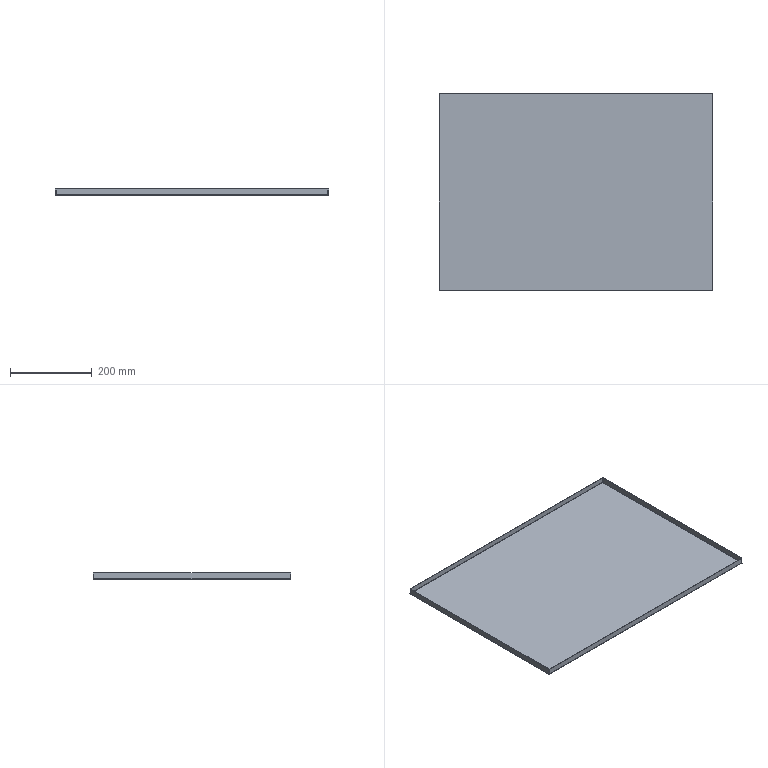Part | SolidWorks | 1 solid | 38 faces | box 670.001 x 485.001 x 15 mm | volume 532568 mm3 | plane 22 | spline 8 | cylinder 8 | commonest cylinder face diameters 0.2 x4 3.2 x4
STEP:
#1=CARTESIAN_POINT('',(333.4,-240.9,-1.5));
#2=VERTEX_POINT('',#1);
#3=CARTESIAN_POINT('',(-333.4,-240.9,-1.5));
#4=VERTEX_POINT('',#3);
#5=CARTESIAN_POINT('',(333.4,-240.9,-1.5));
#6=DIRECTION('',(-1.,0.,0.));
#7=VECTOR('',#6,1000.);
#8=LINE('',#5,#7);
#9=EDGE_CURVE('',#2,#4,#8,.T.);
#10=ORIENTED_EDGE('',*,*,#9,.T.);
#11=CARTESIAN_POINT('',(-333.4,240.9,-1.5));
#12=VERTEX_POINT('',#11);
#13=CARTESIAN_POINT('',(-333.4,-240.9,-1.5));
#14=DIRECTION('',(0.,1.,0.));
#15=VECTOR('',#14,1000.);
#16=LINE('',#13,#15);
#17=EDGE_CURVE('',#4,#12,#16,.T.);
#18=ORIENTED_EDGE('',*,*,#17,.T.);
#19=CARTESIAN_POINT('',(333.4,240.9,-1.5));
#20=VERTEX_POINT('',#19);
#21=CARTESIAN_POINT('',(-333.4,240.9,-1.5));
#22=DIRECTION('',(1.,0.,0.));
#23=VECTOR('',#22,1000.);
#24=LINE('',#21,#23);
#25=EDGE_CURVE('',#12,#20,#24,.T.);
#26=ORIENTED_EDGE('',*,*,#25,.T.);
#27=CARTESIAN_POINT('',(333.4,240.9,-1.5));
#28=DIRECTION('',(0.,-1.,0.));
#29=VECTOR('',#28,1000.);
#30=LINE('',#27,#29);
#31=EDGE_CURVE('',#20,#2,#30,.T.);
#32=ORIENTED_EDGE('',*,*,#31,.T.);
#33=EDGE_LOOP('',(#10,#18,#26,#32));
#34=FACE_OUTER_BOUND('',#33,.T.);
#35=CARTESIAN_POINT('',(0.,0.,-1.5));
#36=DIRECTION('',(0.,0.,1.));
#37=DIRECTION('',(1.,0.,0.));
#38=AXIS2_PLACEMENT_3D('',#35,#36,#37);
#39=PLANE('',#38);
#40=ADVANCED_FACE('',(#34),#39,.F.);
#41=CARTESIAN_POINT('',(-333.4,-240.9,0.));
#42=VERTEX_POINT('',#41);
#43=CARTESIAN_POINT('',(-333.4,240.9,0.));
#44=VERTEX_POINT('',#43);
#45=CARTESIAN_POINT('',(-333.4,-240.9,0.));
#46=DIRECTION('',(0.,1.,0.));
#47=VECTOR('',#46,1000.);
#48=LINE('',#45,#47);
#49=EDGE_CURVE('',#42,#44,#48,.T.);
#50=ORIENTED_EDGE('',*,*,#49,.F.);
#51=CARTESIAN_POINT('',(333.4,-240.9,0.));
#52=VERTEX_POINT('',#51);
#53=CARTESIAN_POINT('',(333.4,-240.9,0.));
#54=DIRECTION('',(-1.,0.,0.));
#55=VECTOR('',#54,1000.);
#56=LINE('',#53,#55);
#57=EDGE_CURVE('',#52,#42,#56,.T.);
#58=ORIENTED_EDGE('',*,*,#57,.F.);
#59=CARTESIAN_POINT('',(333.4,240.9,0.));
#60=VERTEX_POINT('',#59);
#61=CARTESIAN_POINT('',(333.4,240.9,0.));
#62=DIRECTION('',(0.,-1.,0.));
#63=VECTOR('',#62,1000.);
#64=LINE('',#61,#63);
#65=EDGE_CURVE('',#60,#52,#64,.T.);
#66=ORIENTED_EDGE('',*,*,#65,.F.);
#67=CARTESIAN_POINT('',(-333.4,240.9,0.));
#68=DIRECTION('',(1.,0.,0.));
#69=VECTOR('',#68,1000.);
#70=LINE('',#67,#69);
#71=EDGE_CURVE('',#44,#60,#70,.T.);
#72=ORIENTED_EDGE('',*,*,#71,.F.);
#73=EDGE_LOOP('',(#50,#58,#66,#72));
#74=FACE_OUTER_BOUND('',#73,.T.);
#75=CARTESIAN_POINT('',(0.,0.,0.));
#76=DIRECTION('',(0.,0.,1.));
#77=DIRECTION('',(1.,0.,0.));
#78=AXIS2_PLACEMENT_3D('',#75,#76,#77);
#79=PLANE('',#78);
#80=ADVANCED_FACE('',(#74),#79,.T.);
#81=CARTESIAN_POINT('',(-335.,240.293,0.1));
#82=VERTEX_POINT('',#81);
#83=CARTESIAN_POINT('',(-333.5,240.293,0.1));
#84=VERTEX_POINT('',#83);
#85=CARTESIAN_POINT('',(-333.5,240.293,0.1));
#86=DIRECTION('',(1.,0.,0.));
#87=VECTOR('',#86,1000.);
#88=LINE('',#85,#87);
#89=EDGE_CURVE('',#82,#84,#88,.T.);
#90=ORIENTED_EDGE('',*,*,#89,.T.);
#91=CARTESIAN_POINT('',(-333.4,240.9,0.));
#92=CARTESIAN_POINT('',(-333.426,240.799,0.));
#93=CARTESIAN_POINT('',(-333.452,240.698,0.01078));
#94=CARTESIAN_POINT('',(-333.489,240.495,0.0478));
#95=CARTESIAN_POINT('',(-333.5,240.394,0.07382));
#96=CARTESIAN_POINT('',(-333.5,240.293,0.1));
#97=B_SPLINE_CURVE_WITH_KNOTS('',3,(#91,#92,#93,#94,#95,#96),.UNSPECIFIED.,.F.,.F.,(4,2,4),(0.,0.5,1.),.UNSPECIFIED.);
#98=EDGE_CURVE('',#44,#84,#97,.T.);
#99=ORIENTED_EDGE('',*,*,#98,.F.);
#100=CARTESIAN_POINT('',(-333.4,240.9,0.));
#101=DIRECTION('',(0.,0.,-1.));
#102=VECTOR('',#101,1000.);
#103=LINE('',#100,#102);
#104=EDGE_CURVE('',#44,#12,#103,.T.);
#105=ORIENTED_EDGE('',*,*,#104,.T.);
#106=CARTESIAN_POINT('',(-333.4,240.9,-1.5));
#107=CARTESIAN_POINT('',(-333.612,240.849,-1.5));
#108=CARTESIAN_POINT('',(-333.815,240.8,-1.46));
#109=CARTESIAN_POINT('',(-334.205,240.698,-1.299));
#110=CARTESIAN_POINT('',(-334.381,240.648,-1.181));
#111=CARTESIAN_POINT('',(-334.605,240.571,-0.9582));
#112=CARTESIAN_POINT('',(-334.671,240.546,-0.8775));
#113=CARTESIAN_POINT('',(-334.787,240.496,-0.7041));
#114=CARTESIAN_POINT('',(-334.838,240.47,-0.6103));
#115=CARTESIAN_POINT('',(-334.958,240.394,-0.32));
#116=CARTESIAN_POINT('',(-335.,240.344,-0.1115));
#117=CARTESIAN_POINT('',(-335.,240.293,0.1));
#118=B_SPLINE_CURVE_WITH_KNOTS('',3,(#106,#107,#108,#109,#110,#111,#112,#113,#114,#115,#116,#117),.UNSPECIFIED.,.F.,.F.,(4,2,2,2,2,4),(0.,0.0006399,0.00128,0.0016,0.00192,0.00256),.UNSPECIFIED.);
#119=EDGE_CURVE('',#12,#82,#118,.T.);
#120=ORIENTED_EDGE('',*,*,#119,.T.);
#121=EDGE_LOOP('',(#90,#99,#105,#120));
#122=FACE_OUTER_BOUND('',#121,.T.);
#123=CARTESIAN_POINT('',(-333.4,240.9,-1.515));
#124=CARTESIAN_POINT('',(-333.611,240.849,-1.515));
#125=CARTESIAN_POINT('',(-333.823,240.799,-1.473));
#126=CARTESIAN_POINT('',(-334.213,240.698,-1.311));
#127=CARTESIAN_POINT('',(-334.392,240.647,-1.191));
#128=CARTESIAN_POINT('',(-334.691,240.546,-0.8925));
#129=CARTESIAN_POINT('',(-334.811,240.495,-0.7133));
#130=CARTESIAN_POINT('',(-334.973,240.394,-0.3227));
#131=CARTESIAN_POINT('',(-335.015,240.343,-0.1114));
#132=CARTESIAN_POINT('',(-335.015,240.293,0.1));
#133=CARTESIAN_POINT('',(-333.4,240.9,-1.5));
#134=CARTESIAN_POINT('',(-333.609,240.849,-1.5));
#135=CARTESIAN_POINT('',(-333.819,240.799,-1.458));
#136=CARTESIAN_POINT('',(-334.206,240.698,-1.298));
#137=CARTESIAN_POINT('',(-334.383,240.647,-1.179));
#138=CARTESIAN_POINT('',(-334.679,240.546,-0.8833));
#139=CARTESIAN_POINT('',(-334.798,240.495,-0.7058));
#140=CARTESIAN_POINT('',(-334.958,240.394,-0.3188));
#141=CARTESIAN_POINT('',(-335.,240.343,-0.1095));
#142=CARTESIAN_POINT('',(-335.,240.293,0.1));
#143=CARTESIAN_POINT('',(-333.4,240.9,0.));
#144=CARTESIAN_POINT('',(-333.413,240.849,0.));
#145=CARTESIAN_POINT('',(-333.426,240.799,0.002603));
#146=CARTESIAN_POINT('',(-333.45,240.698,0.01262));
#147=CARTESIAN_POINT('',(-333.461,240.647,0.02003));
#148=CARTESIAN_POINT('',(-333.48,240.546,0.03855));
#149=CARTESIAN_POINT('',(-333.487,240.495,0.04964));
#150=CARTESIAN_POINT('',(-333.497,240.394,0.07383));
#151=CARTESIAN_POINT('',(-333.5,240.343,0.08691));
#152=CARTESIAN_POINT('',(-333.5,240.293,0.1));
#153=B_SPLINE_SURFACE_WITH_KNOTS('',1,3,((#123,#124,#125,#126,#127,#128,#129,#130,#131,#132),(#133,#134,#135,#136,#137,#138,#139,#140,#141,#142),(#143,#144,#145,#146,#147,#148,#149,#150,#151,#152)),.UNSPECIFIED.,.F.,.F.,.F.,(2,1,2),(4,2,2,2,4),(-0.01,0.,1.),(0.,0.25,0.5,0.75,1.),.UNSPECIFIED.);
#154=ADVANCED_FACE('',(#122),#153,.F.);
#155=CARTESIAN_POINT('',(-333.5,-240.293,0.1));
#156=VERTEX_POINT('',#155);
#157=CARTESIAN_POINT('',(-333.5,-240.293,0.1));
#158=CARTESIAN_POINT('',(-333.5,-240.394,0.07382));
#159=CARTESIAN_POINT('',(-333.489,-240.495,0.0478));
#160=CARTESIAN_POINT('',(-333.452,-240.698,0.01078));
#161=CARTESIAN_POINT('',(-333.426,-240.799,0.));
#162=CARTESIAN_POINT('',(-333.4,-240.9,0.));
#163=B_SPLINE_CURVE_WITH_KNOTS('',3,(#157,#158,#159,#160,#161,#162),.UNSPECIFIED.,.F.,.F.,(4,2,4),(0.,0.5,1.),.UNSPECIFIED.);
#164=EDGE_CURVE('',#156,#42,#163,.T.);
#165=ORIENTED_EDGE('',*,*,#164,.F.);
#166=CARTESIAN_POINT('',(-335.,-240.293,0.1));
#167=VERTEX_POINT('',#166);
#168=CARTESIAN_POINT('',(-333.5,-240.293,0.1));
#169=DIRECTION('',(1.,0.,0.));
#170=VECTOR('',#169,1000.);
#171=LINE('',#168,#170);
#172=EDGE_CURVE('',#167,#156,#171,.T.);
#173=ORIENTED_EDGE('',*,*,#172,.F.);
#174=CARTESIAN_POINT('',(-335.,-240.293,0.1));
#175=CARTESIAN_POINT('',(-335.,-240.344,-0.1115));
#176=CARTESIAN_POINT('',(-334.96,-240.393,-0.3151));
#177=CARTESIAN_POINT('',(-334.799,-240.495,-0.7048));
#178=CARTESIAN_POINT('',(-334.681,-240.545,-0.881));
#179=CARTESIAN_POINT('',(-334.458,-240.621,-1.105));
#180=CARTESIAN_POINT('',(-334.378,-240.647,-1.171));
#181=CARTESIAN_POINT('',(-334.204,-240.697,-1.287));
#182=CARTESIAN_POINT('',(-334.11,-240.723,-1.338));
#183=CARTESIAN_POINT('',(-333.82,-240.799,-1.458));
#184=CARTESIAN_POINT('',(-333.612,-240.849,-1.5));
#185=CARTESIAN_POINT('',(-333.4,-240.9,-1.5));
#186=B_SPLINE_CURVE_WITH_KNOTS('',3,(#174,#175,#176,#177,#178,#179,#180,#181,#182,#183,#184,#185),.UNSPECIFIED.,.F.,.F.,(4,2,2,2,2,4),(0.,0.0006399,0.00128,0.0016,0.00192,0.00256),.UNSPECIFIED.);
#187=EDGE_CURVE('',#167,#4,#186,.T.);
#188=ORIENTED_EDGE('',*,*,#187,.T.);
#189=CARTESIAN_POINT('',(-333.4,-240.9,0.));
#190=DIRECTION('',(0.,0.,-1.));
#191=VECTOR('',#190,1000.);
#192=LINE('',#189,#191);
#193=EDGE_CURVE('',#42,#4,#192,.T.);
#194=ORIENTED_EDGE('',*,*,#193,.F.);
#195=EDGE_LOOP('',(#165,#173,#188,#194));
#196=FACE_OUTER_BOUND('',#195,.T.);
#197=CARTESIAN_POINT('',(-335.015,-240.293,0.1));
#198=CARTESIAN_POINT('',(-335.015,-240.343,-0.1114));
#199=CARTESIAN_POINT('',(-334.973,-240.394,-0.3227));
#200=CARTESIAN_POINT('',(-334.811,-240.495,-0.7133));
#201=CARTESIAN_POINT('',(-334.691,-240.546,-0.8925));
#202=CARTESIAN_POINT('',(-334.392,-240.647,-1.191));
#203=CARTESIAN_POINT('',(-334.213,-240.698,-1.311));
#204=CARTESIAN_POINT('',(-333.823,-240.799,-1.473));
#205=CARTESIAN_POINT('',(-333.611,-240.849,-1.515));
#206=CARTESIAN_POINT('',(-333.4,-240.9,-1.515));
#207=CARTESIAN_POINT('',(-335.,-240.293,0.1));
#208=CARTESIAN_POINT('',(-335.,-240.343,-0.1095));
#209=CARTESIAN_POINT('',(-334.958,-240.394,-0.3188));
#210=CARTESIAN_POINT('',(-334.798,-240.495,-0.7058));
#211=CARTESIAN_POINT('',(-334.679,-240.546,-0.8833));
#212=CARTESIAN_POINT('',(-334.383,-240.647,-1.179));
#213=CARTESIAN_POINT('',(-334.206,-240.698,-1.298));
#214=CARTESIAN_POINT('',(-333.819,-240.799,-1.458));
#215=CARTESIAN_POINT('',(-333.609,-240.849,-1.5));
#216=CARTESIAN_POINT('',(-333.4,-240.9,-1.5));
#217=CARTESIAN_POINT('',(-333.5,-240.293,0.1));
#218=CARTESIAN_POINT('',(-333.5,-240.343,0.08691));
#219=CARTESIAN_POINT('',(-333.497,-240.394,0.07383));
#220=CARTESIAN_POINT('',(-333.487,-240.495,0.04964));
#221=CARTESIAN_POINT('',(-333.48,-240.546,0.03855));
#222=CARTESIAN_POINT('',(-333.461,-240.647,0.02003));
#223=CARTESIAN_POINT('',(-333.45,-240.698,0.01262));
#224=CARTESIAN_POINT('',(-333.426,-240.799,0.002603));
#225=CARTESIAN_POINT('',(-333.413,-240.849,0.));
#226=CARTESIAN_POINT('',(-333.4,-240.9,0.));
#227=B_SPLINE_SURFACE_WITH_KNOTS('',1,3,((#197,#198,#199,#200,#201,#202,#203,#204,#205,#206),(#207,#208,#209,#210,#211,#212,#213,#214,#215,#216),(#217,#218,#219,#220,#221,#222,#223,#224,#225,#226)),.UNSPECIFIED.,.F.,.F.,.F.,(2,1,2),(4,2,2,2,4),(-0.01,0.,1.),(0.,0.25,0.5,0.75,1.),.UNSPECIFIED.);
#228=ADVANCED_FACE('',(#196),#227,.F.);
#229=ORIENTED_EDGE('',*,*,#17,.F.);
#230=ORIENTED_EDGE('',*,*,#187,.F.);
#231=CARTESIAN_POINT('',(-335.,242.5,0.1));
#232=DIRECTION('',(0.,1.,0.));
#233=VECTOR('',#232,1000.);
#234=LINE('',#231,#233);
#235=EDGE_CURVE('',#167,#82,#234,.T.);
#236=ORIENTED_EDGE('',*,*,#235,.T.);
#237=ORIENTED_EDGE('',*,*,#119,.F.);
#238=EDGE_LOOP('',(#229,#230,#236,#237));
#239=FACE_OUTER_BOUND('',#238,.T.);
#240=CARTESIAN_POINT('',(-333.4,-240.9,0.1));
#241=DIRECTION('',(0.,-1.,0.));
#242=DIRECTION('',(-1.,0.,0.));
#243=AXIS2_PLACEMENT_3D('',#240,#241,#242);
#244=CYLINDRICAL_SURFACE('',#243,1.6);
#245=ADVANCED_FACE('',(#239),#244,.T.);
#246=ORIENTED_EDGE('',*,*,#49,.T.);
#247=ORIENTED_EDGE('',*,*,#98,.T.);
#248=CARTESIAN_POINT('',(-333.5,242.5,0.1));
#249=DIRECTION('',(0.,-1.,0.));
#250=VECTOR('',#249,1000.);
#251=LINE('',#248,#250);
#252=EDGE_CURVE('',#84,#156,#251,.T.);
#253=ORIENTED_EDGE('',*,*,#252,.T.);
#254=ORIENTED_EDGE('',*,*,#164,.T.);
#255=EDGE_LOOP('',(#246,#247,#253,#254));
#256=FACE_OUTER_BOUND('',#255,.T.);
#257=CARTESIAN_POINT('',(-333.4,-240.9,0.1));
#258=DIRECTION('',(0.,-1.,0.));
#259=DIRECTION('',(-1.,0.,0.));
#260=AXIS2_PLACEMENT_3D('',#257,#258,#259);
#261=CYLINDRICAL_SURFACE('',#260,0.1);
#262=ADVANCED_FACE('',(#256),#261,.F.);
#263=CARTESIAN_POINT('',(-335.,240.293,13.5));
#264=VERTEX_POINT('',#263);
#265=CARTESIAN_POINT('',(-335.,240.293,0.));
#266=DIRECTION('',(0.,0.,1.));
#267=VECTOR('',#266,1000.);
#268=LINE('',#265,#267);
#269=EDGE_CURVE('',#82,#264,#268,.T.);
#270=ORIENTED_EDGE('',*,*,#269,.T.);
#271=CARTESIAN_POINT('',(-333.5,240.293,13.5));
#272=VERTEX_POINT('',#271);
#273=CARTESIAN_POINT('',(-333.5,240.293,13.5));
#274=DIRECTION('',(1.,0.,0.));
#275=VECTOR('',#274,1000.);
#276=LINE('',#273,#275);
#277=EDGE_CURVE('',#264,#272,#276,.T.);
#278=ORIENTED_EDGE('',*,*,#277,.T.);
#279=CARTESIAN_POINT('',(-333.5,240.293,0.));
#280=DIRECTION('',(0.,0.,1.));
#281=VECTOR('',#280,1000.);
#282=LINE('',#279,#281);
#283=EDGE_CURVE('',#84,#272,#282,.T.);
#284=ORIENTED_EDGE('',*,*,#283,.F.);
#285=ORIENTED_EDGE('',*,*,#89,.F.);
#286=EDGE_LOOP('',(#270,#278,#284,#285));
#287=FACE_OUTER_BOUND('',#286,.T.);
#288=CARTESIAN_POINT('',(-333.5,240.293,0.));
#289=DIRECTION('',(0.,1.,0.));
#290=DIRECTION('',(0.,0.,1.));
#291=AXIS2_PLACEMENT_3D('',#288,#289,#290);
#292=PLANE('',#291);
#293=ADVANCED_FACE('',(#287),#292,.T.);
#294=ORIENTED_EDGE('',*,*,#235,.F.);
#295=CARTESIAN_POINT('',(-335.,-240.293,13.5));
#296=VERTEX_POINT('',#295);
#297=CARTESIAN_POINT('',(-335.,-240.293,0.));
#298=DIRECTION('',(0.,0.,1.));
#299=VECTOR('',#298,1000.);
#300=LINE('',#297,#299);
#301=EDGE_CURVE('',#167,#296,#300,.T.);
#302=ORIENTED_EDGE('',*,*,#301,.T.);
#303=CARTESIAN_POINT('',(-335.,0.,13.5));
#304=DIRECTION('',(0.,1.,0.));
#305=VECTOR('',#304,1000.);
#306=LINE('',#303,#305);
#307=EDGE_CURVE('',#296,#264,#306,.T.);
#308=ORIENTED_EDGE('',*,*,#307,.T.);
#309=ORIENTED_EDGE('',*,*,#269,.F.);
#310=EDGE_LOOP('',(#294,#302,#308,#309));
#311=FACE_OUTER_BOUND('',#310,.T.);
#312=CARTESIAN_POINT('',(-335.,0.,0.));
#313=DIRECTION('',(1.,0.,0.));
#314=DIRECTION('',(0.,0.,-1.));
#315=AXIS2_PLACEMENT_3D('',#312,#313,#314);
#316=PLANE('',#315);
#317=ADVANCED_FACE('',(#311),#316,.F.);
#318=CARTESIAN_POINT('',(-333.5,-240.293,13.5));
#319=VERTEX_POINT('',#318);
#320=CARTESIAN_POINT('',(-333.5,-240.293,0.));
#321=DIRECTION('',(0.,0.,1.));
#322=VECTOR('',#321,1000.);
#323=LINE('',#320,#322);
#324=EDGE_CURVE('',#156,#319,#323,.T.);
#325=ORIENTED_EDGE('',*,*,#324,.F.);
#326=ORIENTED_EDGE('',*,*,#252,.F.);
#327=ORIENTED_EDGE('',*,*,#283,.T.);
#328=CARTESIAN_POINT('',(-333.5,242.5,13.5));
#329=DIRECTION('',(0.,1.,0.));
#330=VECTOR('',#329,1000.);
#331=LINE('',#328,#330);
#332=EDGE_CURVE('',#319,#272,#331,.T.);
#333=ORIENTED_EDGE('',*,*,#332,.F.);
#334=EDGE_LOOP('',(#325,#326,#327,#333));
#335=FACE_OUTER_BOUND('',#334,.T.);
#336=CARTESIAN_POINT('',(-333.5,0.,0.));
#337=DIRECTION('',(1.,0.,0.));
#338=DIRECTION('',(0.,0.,-1.));
#339=AXIS2_PLACEMENT_3D('',#336,#337,#338);
#340=PLANE('',#339);
#341=ADVANCED_FACE('',(#335),#340,.T.);
#342=ORIENTED_EDGE('',*,*,#307,.F.);
#343=CARTESIAN_POINT('',(-335.,-240.293,13.5));
#344=DIRECTION('',(1.,0.,0.));
#345=VECTOR('',#344,1000.);
#346=LINE('',#343,#345);
#347=EDGE_CURVE('',#296,#319,#346,.T.);
#348=ORIENTED_EDGE('',*,*,#347,.T.);
#349=ORIENTED_EDGE('',*,*,#332,.T.);
#350=ORIENTED_EDGE('',*,*,#277,.F.);
#351=EDGE_LOOP('',(#342,#348,#349,#350));
#352=FACE_OUTER_BOUND('',#351,.T.);
#353=CARTESIAN_POINT('',(-335.,242.5,13.5));
#354=DIRECTION('',(0.,0.,-1.));
#355=DIRECTION('',(-1.,0.,0.));
#356=AXIS2_PLACEMENT_3D('',#353,#354,#355);
#357=PLANE('',#356);
#358=ADVANCED_FACE('',(#352),#357,.F.);
#359=ORIENTED_EDGE('',*,*,#347,.F.);
#360=ORIENTED_EDGE('',*,*,#301,.F.);
#361=ORIENTED_EDGE('',*,*,#172,.T.);
#362=ORIENTED_EDGE('',*,*,#324,.T.);
#363=EDGE_LOOP('',(#359,#360,#361,#362));
#364=FACE_OUTER_BOUND('',#363,.T.);
#365=CARTESIAN_POINT('',(-333.5,-240.293,0.));
#366=DIRECTION('',(0.,1.,0.));
#367=DIRECTION('',(0.,0.,1.));
#368=AXIS2_PLACEMENT_3D('',#365,#366,#367);
#369=PLANE('',#368);
#370=ADVANCED_FACE('',(#364),#369,.F.);
#371=CARTESIAN_POINT('',(332.793,242.5,0.1));
#372=VERTEX_POINT('',#371);
#373=CARTESIAN_POINT('',(332.793,241.,0.1));
#374=VERTEX_POINT('',#373);
#375=CARTESIAN_POINT('',(332.793,241.,0.1));
#376=DIRECTION('',(0.,-1.,0.));
#377=VECTOR('',#376,1000.);
#378=LINE('',#375,#377);
#379=EDGE_CURVE('',#372,#374,#378,.T.);
#380=ORIENTED_EDGE('',*,*,#379,.T.);
#381=CARTESIAN_POINT('',(333.4,240.9,0.));
#382=CARTESIAN_POINT('',(333.299,240.926,0.));
#383=CARTESIAN_POINT('',(333.198,240.952,0.01078));
#384=CARTESIAN_POINT('',(332.995,240.989,0.0478));
#385=CARTESIAN_POINT('',(332.894,241.,0.07382));
#386=CARTESIAN_POINT('',(332.793,241.,0.1));
#387=B_SPLINE_CURVE_WITH_KNOTS('',3,(#381,#382,#383,#384,#385,#386),.UNSPECIFIED.,.F.,.F.,(4,2,4),(0.,0.5,1.),.UNSPECIFIED.);
#388=EDGE_CURVE('',#60,#374,#387,.T.);
#389=ORIENTED_EDGE('',*,*,#388,.F.);
#390=CARTESIAN_POINT('',(333.4,240.9,0.));
#391=DIRECTION('',(0.,0.,-1.));
#392=VECTOR('',#391,1000.);
#393=LINE('',#390,#392);
#394=EDGE_CURVE('',#60,#20,#393,.T.);
#395=ORIENTED_EDGE('',*,*,#394,.T.);
#396=CARTESIAN_POINT('',(333.4,240.9,-1.5));
#397=CARTESIAN_POINT('',(333.349,241.112,-1.5));
#398=CARTESIAN_POINT('',(333.3,241.315,-1.46));
#399=CARTESIAN_POINT('',(333.198,241.705,-1.299));
#400=CARTESIAN_POINT('',(333.148,241.881,-1.181));
#401=CARTESIAN_POINT('',(333.071,242.105,-0.9582));
#402=CARTESIAN_POINT('',(333.046,242.171,-0.8775));
#403=CARTESIAN_POINT('',(332.996,242.287,-0.7041));
#404=CARTESIAN_POINT('',(332.97,242.338,-0.6103));
#405=CARTESIAN_POINT('',(332.894,242.458,-0.32));
#406=CARTESIAN_POINT('',(332.844,242.5,-0.1115));
#407=CARTESIAN_POINT('',(332.793,242.5,0.1));
#408=B_SPLINE_CURVE_WITH_KNOTS('',3,(#396,#397,#398,#399,#400,#401,#402,#403,#404,#405,#406,#407),.UNSPECIFIED.,.F.,.F.,(4,2,2,2,2,4),(0.,0.0006399,0.00128,0.0016,0.00192,0.00256),.UNSPECIFIED.);
#409=EDGE_CURVE('',#20,#372,#408,.T.);
#410=ORIENTED_EDGE('',*,*,#409,.T.);
#411=EDGE_LOOP('',(#380,#389,#395,#410));
#412=FACE_OUTER_BOUND('',#411,.T.);
#413=CARTESIAN_POINT('',(333.4,240.9,-1.515));
#414=CARTESIAN_POINT('',(333.349,241.111,-1.515));
#415=CARTESIAN_POINT('',(333.299,241.323,-1.473));
#416=CARTESIAN_POINT('',(333.198,241.713,-1.311));
#417=CARTESIAN_POINT('',(333.147,241.892,-1.191));
#418=CARTESIAN_POINT('',(333.046,242.191,-0.8925));
#419=CARTESIAN_POINT('',(332.995,242.311,-0.7133));
#420=CARTESIAN_POINT('',(332.894,242.473,-0.3227));
#421=CARTESIAN_POINT('',(332.843,242.515,-0.1114));
#422=CARTESIAN_POINT('',(332.793,242.515,0.1));
#423=CARTESIAN_POINT('',(333.4,240.9,-1.5));
#424=CARTESIAN_POINT('',(333.349,241.109,-1.5));
#425=CARTESIAN_POINT('',(333.299,241.319,-1.458));
#426=CARTESIAN_POINT('',(333.198,241.706,-1.298));
#427=CARTESIAN_POINT('',(333.147,241.883,-1.179));
#428=CARTESIAN_POINT('',(333.046,242.179,-0.8833));
#429=CARTESIAN_POINT('',(332.995,242.298,-0.7058));
#430=CARTESIAN_POINT('',(332.894,242.458,-0.3188));
#431=CARTESIAN_POINT('',(332.843,242.5,-0.1095));
#432=CARTESIAN_POINT('',(332.793,242.5,0.1));
#433=CARTESIAN_POINT('',(333.4,240.9,0.));
#434=CARTESIAN_POINT('',(333.349,240.913,0.));
#435=CARTESIAN_POINT('',(333.299,240.926,0.002603));
#436=CARTESIAN_POINT('',(333.198,240.95,0.01262));
#437=CARTESIAN_POINT('',(333.147,240.961,0.02003));
#438=CARTESIAN_POINT('',(333.046,240.98,0.03855));
#439=CARTESIAN_POINT('',(332.995,240.987,0.04964));
#440=CARTESIAN_POINT('',(332.894,240.997,0.07383));
#441=CARTESIAN_POINT('',(332.843,241.,0.08691));
#442=CARTESIAN_POINT('',(332.793,241.,0.1));
#443=B_SPLINE_SURFACE_WITH_KNOTS('',1,3,((#413,#414,#415,#416,#417,#418,#419,#420,#421,#422),(#423,#424,#425,#426,#427,#428,#429,#430,#431,#432),(#433,#434,#435,#436,#437,#438,#439,#440,#441,#442)),.UNSPECIFIED.,.F.,.F.,.F.,(2,1,2),(4,2,2,2,4),(-0.01,0.,1.),(0.,0.25,0.5,0.75,1.),.UNSPECIFIED.);
#444=ADVANCED_FACE('',(#412),#443,.F.);
#445=CARTESIAN_POINT('',(-332.793,241.,0.1));
#446=VERTEX_POINT('',#445);
#447=CARTESIAN_POINT('',(-332.793,241.,0.1));
#448=CARTESIAN_POINT('',(-332.894,241.,0.07382));
#449=CARTESIAN_POINT('',(-332.995,240.989,0.0478));
#450=CARTESIAN_POINT('',(-333.198,240.952,0.01078));
#451=CARTESIAN_POINT('',(-333.299,240.926,0.));
#452=CARTESIAN_POINT('',(-333.4,240.9,0.));
#453=B_SPLINE_CURVE_WITH_KNOTS('',3,(#447,#448,#449,#450,#451,#452),.UNSPECIFIED.,.F.,.F.,(4,2,4),(0.,0.5,1.),.UNSPECIFIED.);
#454=EDGE_CURVE('',#446,#44,#453,.T.);
#455=ORIENTED_EDGE('',*,*,#454,.F.);
#456=CARTESIAN_POINT('',(-332.793,242.5,0.1));
#457=VERTEX_POINT('',#456);
#458=CARTESIAN_POINT('',(-332.793,241.,0.1));
#459=DIRECTION('',(0.,-1.,0.));
#460=VECTOR('',#459,1000.);
#461=LINE('',#458,#460);
#462=EDGE_CURVE('',#457,#446,#461,.T.);
#463=ORIENTED_EDGE('',*,*,#462,.F.);
#464=CARTESIAN_POINT('',(-332.793,242.5,0.1));
#465=CARTESIAN_POINT('',(-332.844,242.5,-0.1115));
#466=CARTESIAN_POINT('',(-332.893,242.46,-0.3151));
#467=CARTESIAN_POINT('',(-332.995,242.299,-0.7048));
#468=CARTESIAN_POINT('',(-333.045,242.181,-0.881));
#469=CARTESIAN_POINT('',(-333.121,241.958,-1.105));
#470=CARTESIAN_POINT('',(-333.147,241.878,-1.171));
#471=CARTESIAN_POINT('',(-333.197,241.704,-1.287));
#472=CARTESIAN_POINT('',(-333.223,241.61,-1.338));
#473=CARTESIAN_POINT('',(-333.299,241.32,-1.458));
#474=CARTESIAN_POINT('',(-333.349,241.112,-1.5));
#475=CARTESIAN_POINT('',(-333.4,240.9,-1.5));
#476=B_SPLINE_CURVE_WITH_KNOTS('',3,(#464,#465,#466,#467,#468,#469,#470,#471,#472,#473,#474,#475),.UNSPECIFIED.,.F.,.F.,(4,2,2,2,2,4),(0.,0.0006399,0.00128,0.0016,0.00192,0.00256),.UNSPECIFIED.);
#477=EDGE_CURVE('',#457,#12,#476,.T.);
#478=ORIENTED_EDGE('',*,*,#477,.T.);
#479=ORIENTED_EDGE('',*,*,#104,.F.);
#480=EDGE_LOOP('',(#455,#463,#478,#479));
#481=FACE_OUTER_BOUND('',#480,.T.);
#482=CARTESIAN_POINT('',(-332.793,242.515,0.1));
#483=CARTESIAN_POINT('',(-332.843,242.515,-0.1114));
#484=CARTESIAN_POINT('',(-332.894,242.473,-0.3227));
#485=CARTESIAN_POINT('',(-332.995,242.311,-0.7133));
#486=CARTESIAN_POINT('',(-333.046,242.191,-0.8925));
#487=CARTESIAN_POINT('',(-333.147,241.892,-1.191));
#488=CARTESIAN_POINT('',(-333.198,241.713,-1.311));
#489=CARTESIAN_POINT('',(-333.299,241.323,-1.473));
#490=CARTESIAN_POINT('',(-333.349,241.111,-1.515));
#491=CARTESIAN_POINT('',(-333.4,240.9,-1.515));
#492=CARTESIAN_POINT('',(-332.793,242.5,0.1));
#493=CARTESIAN_POINT('',(-332.843,242.5,-0.1095));
#494=CARTESIAN_POINT('',(-332.894,242.458,-0.3188));
#495=CARTESIAN_POINT('',(-332.995,242.298,-0.7058));
#496=CARTESIAN_POINT('',(-333.046,242.179,-0.8833));
#497=CARTESIAN_POINT('',(-333.147,241.883,-1.179));
#498=CARTESIAN_POINT('',(-333.198,241.706,-1.298));
#499=CARTESIAN_POINT('',(-333.299,241.319,-1.458));
#500=CARTESIAN_POINT('',(-333.349,241.109,-1.5));
#501=CARTESIAN_POINT('',(-333.4,240.9,-1.5));
#502=CARTESIAN_POINT('',(-332.793,241.,0.1));
#503=CARTESIAN_POINT('',(-332.843,241.,0.08691));
#504=CARTESIAN_POINT('',(-332.894,240.997,0.07383));
#505=CARTESIAN_POINT('',(-332.995,240.987,0.04964));
#506=CARTESIAN_POINT('',(-333.046,240.98,0.03855));
#507=CARTESIAN_POINT('',(-333.147,240.961,0.02003));
#508=CARTESIAN_POINT('',(-333.198,240.95,0.01262));
#509=CARTESIAN_POINT('',(-333.299,240.926,0.002603));
#510=CARTESIAN_POINT('',(-333.349,240.913,0.));
#511=CARTESIAN_POINT('',(-333.4,240.9,0.));
#512=B_SPLINE_SURFACE_WITH_KNOTS('',1,3,((#482,#483,#484,#485,#486,#487,#488,#489,#490,#491),(#492,#493,#494,#495,#496,#497,#498,#499,#500,#501),(#502,#503,#504,#505,#506,#507,#508,#509,#510,#511)),.UNSPECIFIED.,.F.,.F.,.F.,(2,1,2),(4,2,2,2,4),(-0.01,0.,1.),(0.,0.25,0.5,0.75,1.),.UNSPECIFIED.);
#513=ADVANCED_FACE('',(#481),#512,.F.);
#514=ORIENTED_EDGE('',*,*,#25,.F.);
#515=ORIENTED_EDGE('',*,*,#477,.F.);
#516=CARTESIAN_POINT('',(335.,242.5,0.1));
#517=DIRECTION('',(1.,0.,0.));
#518=VECTOR('',#517,1000.);
#519=LINE('',#516,#518);
#520=EDGE_CURVE('',#457,#372,#519,.T.);
#521=ORIENTED_EDGE('',*,*,#520,.T.);
#522=ORIENTED_EDGE('',*,*,#409,.F.);
#523=EDGE_LOOP('',(#514,#515,#521,#522));
#524=FACE_OUTER_BOUND('',#523,.T.);
#525=CARTESIAN_POINT('',(-333.4,240.9,0.1));
#526=DIRECTION('',(-1.,0.,0.));
#527=DIRECTION('',(0.,1.,0.));
#528=AXIS2_PLACEMENT_3D('',#525,#526,#527);
#529=CYLINDRICAL_SURFACE('',#528,1.6);
#530=ADVANCED_FACE('',(#524),#529,.T.);
#531=ORIENTED_EDGE('',*,*,#71,.T.);
#532=ORIENTED_EDGE('',*,*,#388,.T.);
#533=CARTESIAN_POINT('',(335.,241.,0.1));
#534=DIRECTION('',(-1.,0.,0.));
#535=VECTOR('',#534,1000.);
#536=LINE('',#533,#535);
#537=EDGE_CURVE('',#374,#446,#536,.T.);
#538=ORIENTED_EDGE('',*,*,#537,.T.);
#539=ORIENTED_EDGE('',*,*,#454,.T.);
#540=EDGE_LOOP('',(#531,#532,#538,#539));
#541=FACE_OUTER_BOUND('',#540,.T.);
#542=CARTESIAN_POINT('',(-333.4,240.9,0.1));
#543=DIRECTION('',(-1.,0.,0.));
#544=DIRECTION('',(0.,1.,0.));
#545=AXIS2_PLACEMENT_3D('',#542,#543,#544);
#546=CYLINDRICAL_SURFACE('',#545,0.1);
#547=ADVANCED_FACE('',(#541),#546,.F.);
#548=CARTESIAN_POINT('',(332.793,242.5,13.5));
#549=VERTEX_POINT('',#548);
#550=CARTESIAN_POINT('',(332.793,242.5,0.));
#551=DIRECTION('',(0.,0.,1.));
#552=VECTOR('',#551,1000.);
#553=LINE('',#550,#552);
#554=EDGE_CURVE('',#372,#549,#553,.T.);
#555=ORIENTED_EDGE('',*,*,#554,.T.);
#556=CARTESIAN_POINT('',(332.793,241.,13.5));
#557=VERTEX_POINT('',#556);
#558=CARTESIAN_POINT('',(332.793,241.,13.5));
#559=DIRECTION('',(0.,-1.,0.));
#560=VECTOR('',#559,1000.);
#561=LINE('',#558,#560);
#562=EDGE_CURVE('',#549,#557,#561,.T.);
#563=ORIENTED_EDGE('',*,*,#562,.T.);
#564=CARTESIAN_POINT('',(332.793,241.,0.));
#565=DIRECTION('',(0.,0.,1.));
#566=VECTOR('',#565,1000.);
#567=LINE('',#564,#566);
#568=EDGE_CURVE('',#374,#557,#567,.T.);
#569=ORIENTED_EDGE('',*,*,#568,.F.);
#570=ORIENTED_EDGE('',*,*,#379,.F.);
#571=EDGE_LOOP('',(#555,#563,#569,#570));
#572=FACE_OUTER_BOUND('',#571,.T.);
#573=CARTESIAN_POINT('',(332.793,241.,0.));
#574=DIRECTION('',(1.,0.,0.));
#575=DIRECTION('',(0.,0.,-1.));
#576=AXIS2_PLACEMENT_3D('',#573,#574,#575);
#577=PLANE('',#576);
#578=ADVANCED_FACE('',(#572),#577,.T.);
#579=ORIENTED_EDGE('',*,*,#520,.F.);
#580=CARTESIAN_POINT('',(-332.793,242.5,13.5));
#581=VERTEX_POINT('',#580);
#582=CARTESIAN_POINT('',(-332.793,242.5,0.));
#583=DIRECTION('',(0.,0.,1.));
#584=VECTOR('',#583,1000.);
#585=LINE('',#582,#584);
#586=EDGE_CURVE('',#457,#581,#585,.T.);
#587=ORIENTED_EDGE('',*,*,#586,.T.);
#588=CARTESIAN_POINT('',(0.,242.5,13.5));
#589=DIRECTION('',(1.,0.,0.));
#590=VECTOR('',#589,1000.);
#591=LINE('',#588,#590);
#592=EDGE_CURVE('',#581,#549,#591,.T.);
#593=ORIENTED_EDGE('',*,*,#592,.T.);
#594=ORIENTED_EDGE('',*,*,#554,.F.);
#595=EDGE_LOOP('',(#579,#587,#593,#594));
#596=FACE_OUTER_BOUND('',#595,.T.);
#597=CARTESIAN_POINT('',(0.,242.5,0.));
#598=DIRECTION('',(0.,-1.,0.));
#599=DIRECTION('',(0.,0.,-1.));
#600=AXIS2_PLACEMENT_3D('',#597,#598,#599);
#601=PLANE('',#600);
#602=ADVANCED_FACE('',(#596),#601,.F.);
#603=CARTESIAN_POINT('',(-332.793,241.,13.5));
#604=VERTEX_POINT('',#603);
#605=CARTESIAN_POINT('',(-332.793,241.,0.));
#606=DIRECTION('',(0.,0.,1.));
#607=VECTOR('',#606,1000.);
#608=LINE('',#605,#607);
#609=EDGE_CURVE('',#446,#604,#608,.T.);
#610=ORIENTED_EDGE('',*,*,#609,.F.);
#611=ORIENTED_EDGE('',*,*,#537,.F.);
#612=ORIENTED_EDGE('',*,*,#568,.T.);
#613=CARTESIAN_POINT('',(335.,241.,13.5));
#614=DIRECTION('',(1.,0.,0.));
#615=VECTOR('',#614,1000.);
#616=LINE('',#613,#615);
#617=EDGE_CURVE('',#604,#557,#616,.T.);
#618=ORIENTED_EDGE('',*,*,#617,.F.);
#619=EDGE_LOOP('',(#610,#611,#612,#618));
#620=FACE_OUTER_BOUND('',#619,.T.);
#621=CARTESIAN_POINT('',(0.,241.,0.));
#622=DIRECTION('',(0.,-1.,0.));
#623=DIRECTION('',(0.,0.,-1.));
#624=AXIS2_PLACEMENT_3D('',#621,#622,#623);
#625=PLANE('',#624);
#626=ADVANCED_FACE('',(#620),#625,.T.);
#627=ORIENTED_EDGE('',*,*,#592,.F.);
#628=CARTESIAN_POINT('',(-332.793,242.5,13.5));
#629=DIRECTION('',(0.,-1.,0.));
#630=VECTOR('',#629,1000.);
#631=LINE('',#628,#630);
#632=EDGE_CURVE('',#581,#604,#631,.T.);
#633=ORIENTED_EDGE('',*,*,#632,.T.);
#634=ORIENTED_EDGE('',*,*,#617,.T.);
#635=ORIENTED_EDGE('',*,*,#562,.F.);
#636=EDGE_LOOP('',(#627,#633,#634,#635));
#637=FACE_OUTER_BOUND('',#636,.T.);
#638=CARTESIAN_POINT('',(335.,242.5,13.5));
#639=DIRECTION('',(0.,0.,-1.));
#640=DIRECTION('',(0.,1.,0.));
#641=AXIS2_PLACEMENT_3D('',#638,#639,#640);
#642=PLANE('',#641);
#643=ADVANCED_FACE('',(#637),#642,.F.);
#644=ORIENTED_EDGE('',*,*,#632,.F.);
#645=ORIENTED_EDGE('',*,*,#586,.F.);
#646=ORIENTED_EDGE('',*,*,#462,.T.);
#647=ORIENTED_EDGE('',*,*,#609,.T.);
#648=EDGE_LOOP('',(#644,#645,#646,#647));
#649=FACE_OUTER_BOUND('',#648,.T.);
#650=CARTESIAN_POINT('',(-332.793,241.,0.));
#651=DIRECTION('',(1.,0.,0.));
#652=DIRECTION('',(0.,0.,-1.));
#653=AXIS2_PLACEMENT_3D('',#650,#651,#652);
#654=PLANE('',#653);
#655=ADVANCED_FACE('',(#649),#654,.F.);
#656=CARTESIAN_POINT('',(335.,-240.293,0.1));
#657=VERTEX_POINT('',#656);
#658=CARTESIAN_POINT('',(333.5,-240.293,0.1));
#659=VERTEX_POINT('',#658);
#660=CARTESIAN_POINT('',(333.5,-240.293,0.1));
#661=DIRECTION('',(-1.,0.,0.));
#662=VECTOR('',#661,1000.);
#663=LINE('',#660,#662);
#664=EDGE_CURVE('',#657,#659,#663,.T.);
#665=ORIENTED_EDGE('',*,*,#664,.T.);
#666=CARTESIAN_POINT('',(333.4,-240.9,0.));
#667=CARTESIAN_POINT('',(333.426,-240.799,0.));
#668=CARTESIAN_POINT('',(333.452,-240.698,0.01078));
#669=CARTESIAN_POINT('',(333.489,-240.495,0.0478));
#670=CARTESIAN_POINT('',(333.5,-240.394,0.07382));
#671=CARTESIAN_POINT('',(333.5,-240.293,0.1));
#672=B_SPLINE_CURVE_WITH_KNOTS('',3,(#666,#667,#668,#669,#670,#671),.UNSPECIFIED.,.F.,.F.,(4,2,4),(0.,0.5,1.),.UNSPECIFIED.);
#673=EDGE_CURVE('',#52,#659,#672,.T.);
#674=ORIENTED_EDGE('',*,*,#673,.F.);
#675=CARTESIAN_POINT('',(333.4,-240.9,0.));
#676=DIRECTION('',(0.,0.,-1.));
#677=VECTOR('',#676,1000.);
#678=LINE('',#675,#677);
#679=EDGE_CURVE('',#52,#2,#678,.T.);
#680=ORIENTED_EDGE('',*,*,#679,.T.);
#681=CARTESIAN_POINT('',(333.4,-240.9,-1.5));
#682=CARTESIAN_POINT('',(333.612,-240.849,-1.5));
#683=CARTESIAN_POINT('',(333.815,-240.8,-1.46));
#684=CARTESIAN_POINT('',(334.205,-240.698,-1.299));
#685=CARTESIAN_POINT('',(334.381,-240.648,-1.181));
#686=CARTESIAN_POINT('',(334.605,-240.571,-0.9582));
#687=CARTESIAN_POINT('',(334.671,-240.546,-0.8775));
#688=CARTESIAN_POINT('',(334.787,-240.496,-0.7041));
#689=CARTESIAN_POINT('',(334.838,-240.47,-0.6103));
#690=CARTESIAN_POINT('',(334.958,-240.394,-0.32));
#691=CARTESIAN_POINT('',(335.,-240.344,-0.1115));
#692=CARTESIAN_POINT('',(335.,-240.293,0.1));
#693=B_SPLINE_CURVE_WITH_KNOTS('',3,(#681,#682,#683,#684,#685,#686,#687,#688,#689,#690,#691,#692),.UNSPECIFIED.,.F.,.F.,(4,2,2,2,2,4),(0.,0.0006399,0.00128,0.0016,0.00192,0.00256),.UNSPECIFIED.);
#694=EDGE_CURVE('',#2,#657,#693,.T.);
#695=ORIENTED_EDGE('',*,*,#694,.T.);
#696=EDGE_LOOP('',(#665,#674,#680,#695));
#697=FACE_OUTER_BOUND('',#696,.T.);
#698=CARTESIAN_POINT('',(333.4,-240.9,-1.515));
#699=CARTESIAN_POINT('',(333.611,-240.849,-1.515));
#700=CARTESIAN_POINT('',(333.823,-240.799,-1.473));
#701=CARTESIAN_POINT('',(334.213,-240.698,-1.311));
#702=CARTESIAN_POINT('',(334.392,-240.647,-1.191));
#703=CARTESIAN_POINT('',(334.691,-240.546,-0.8925));
#704=CARTESIAN_POINT('',(334.811,-240.495,-0.7133));
#705=CARTESIAN_POINT('',(334.973,-240.394,-0.3227));
#706=CARTESIAN_POINT('',(335.015,-240.343,-0.1114));
#707=CARTESIAN_POINT('',(335.015,-240.293,0.1));
#708=CARTESIAN_POINT('',(333.4,-240.9,-1.5));
#709=CARTESIAN_POINT('',(333.609,-240.849,-1.5));
#710=CARTESIAN_POINT('',(333.819,-240.799,-1.458));
#711=CARTESIAN_POINT('',(334.206,-240.698,-1.298));
#712=CARTESIAN_POINT('',(334.383,-240.647,-1.179));
#713=CARTESIAN_POINT('',(334.679,-240.546,-0.8833));
#714=CARTESIAN_POINT('',(334.798,-240.495,-0.7058));
#715=CARTESIAN_POINT('',(334.958,-240.394,-0.3188));
#716=CARTESIAN_POINT('',(335.,-240.343,-0.1095));
#717=CARTESIAN_POINT('',(335.,-240.293,0.1));
#718=CARTESIAN_POINT('',(333.4,-240.9,0.));
#719=CARTESIAN_POINT('',(333.413,-240.849,0.));
#720=CARTESIAN_POINT('',(333.426,-240.799,0.002603));
#721=CARTESIAN_POINT('',(333.45,-240.698,0.01262));
#722=CARTESIAN_POINT('',(333.461,-240.647,0.02003));
#723=CARTESIAN_POINT('',(333.48,-240.546,0.03855));
#724=CARTESIAN_POINT('',(333.487,-240.495,0.04964));
#725=CARTESIAN_POINT('',(333.497,-240.394,0.07383));
#726=CARTESIAN_POINT('',(333.5,-240.343,0.08691));
#727=CARTESIAN_POINT('',(333.5,-240.293,0.1));
#728=B_SPLINE_SURFACE_WITH_KNOTS('',1,3,((#698,#699,#700,#701,#702,#703,#704,#705,#706,#707),(#708,#709,#710,#711,#712,#713,#714,#715,#716,#717),(#718,#719,#720,#721,#722,#723,#724,#725,#726,#727)),.UNSPECIFIED.,.F.,.F.,.F.,(2,1,2),(4,2,2,2,4),(-0.01,0.,1.),(0.,0.25,0.5,0.75,1.),.UNSPECIFIED.);
#729=ADVANCED_FACE('',(#697),#728,.F.);
#730=CARTESIAN_POINT('',(333.5,240.293,0.1));
#731=VERTEX_POINT('',#730);
#732=CARTESIAN_POINT('',(333.5,240.293,0.1));
#733=CARTESIAN_POINT('',(333.5,240.394,0.07382));
#734=CARTESIAN_POINT('',(333.489,240.495,0.0478));
#735=CARTESIAN_POINT('',(333.452,240.698,0.01078));
#736=CARTESIAN_POINT('',(333.426,240.799,0.));
#737=CARTESIAN_POINT('',(333.4,240.9,0.));
#738=B_SPLINE_CURVE_WITH_KNOTS('',3,(#732,#733,#734,#735,#736,#737),.UNSPECIFIED.,.F.,.F.,(4,2,4),(0.,0.5,1.),.UNSPECIFIED.);
#739=EDGE_CURVE('',#731,#60,#738,.T.);
#740=ORIENTED_EDGE('',*,*,#739,.F.);
#741=CARTESIAN_POINT('',(335.,240.293,0.1));
#742=VERTEX_POINT('',#741);
#743=CARTESIAN_POINT('',(333.5,240.293,0.1));
#744=DIRECTION('',(-1.,0.,0.));
#745=VECTOR('',#744,1000.);
#746=LINE('',#743,#745);
#747=EDGE_CURVE('',#742,#731,#746,.T.);
#748=ORIENTED_EDGE('',*,*,#747,.F.);
#749=CARTESIAN_POINT('',(335.,240.293,0.1));
#750=CARTESIAN_POINT('',(335.,240.344,-0.1115));
#751=CARTESIAN_POINT('',(334.96,240.393,-0.3151));
#752=CARTESIAN_POINT('',(334.799,240.495,-0.7048));
#753=CARTESIAN_POINT('',(334.681,240.545,-0.881));
#754=CARTESIAN_POINT('',(334.458,240.621,-1.105));
#755=CARTESIAN_POINT('',(334.378,240.647,-1.171));
#756=CARTESIAN_POINT('',(334.204,240.697,-1.287));
#757=CARTESIAN_POINT('',(334.11,240.723,-1.338));
#758=CARTESIAN_POINT('',(333.82,240.799,-1.458));
#759=CARTESIAN_POINT('',(333.612,240.849,-1.5));
#760=CARTESIAN_POINT('',(333.4,240.9,-1.5));
#761=B_SPLINE_CURVE_WITH_KNOTS('',3,(#749,#750,#751,#752,#753,#754,#755,#756,#757,#758,#759,#760),.UNSPECIFIED.,.F.,.F.,(4,2,2,2,2,4),(0.,0.0006399,0.00128,0.0016,0.00192,0.00256),.UNSPECIFIED.);
#762=EDGE_CURVE('',#742,#20,#761,.T.);
#763=ORIENTED_EDGE('',*,*,#762,.T.);
#764=ORIENTED_EDGE('',*,*,#394,.F.);
#765=EDGE_LOOP('',(#740,#748,#763,#764));
#766=FACE_OUTER_BOUND('',#765,.T.);
#767=CARTESIAN_POINT('',(335.015,240.293,0.1));
#768=CARTESIAN_POINT('',(335.015,240.343,-0.1114));
#769=CARTESIAN_POINT('',(334.973,240.394,-0.3227));
#770=CARTESIAN_POINT('',(334.811,240.495,-0.7133));
#771=CARTESIAN_POINT('',(334.691,240.546,-0.8925));
#772=CARTESIAN_POINT('',(334.392,240.647,-1.191));
#773=CARTESIAN_POINT('',(334.213,240.698,-1.311));
#774=CARTESIAN_POINT('',(333.823,240.799,-1.473));
#775=CARTESIAN_POINT('',(333.611,240.849,-1.515));
#776=CARTESIAN_POINT('',(333.4,240.9,-1.515));
#777=CARTESIAN_POINT('',(335.,240.293,0.1));
#778=CARTESIAN_POINT('',(335.,240.343,-0.1095));
#779=CARTESIAN_POINT('',(334.958,240.394,-0.3188));
#780=CARTESIAN_POINT('',(334.798,240.495,-0.7058));
#781=CARTESIAN_POINT('',(334.679,240.546,-0.8833));
#782=CARTESIAN_POINT('',(334.383,240.647,-1.179));
#783=CARTESIAN_POINT('',(334.206,240.698,-1.298));
#784=CARTESIAN_POINT('',(333.819,240.799,-1.458));
#785=CARTESIAN_POINT('',(333.609,240.849,-1.5));
#786=CARTESIAN_POINT('',(333.4,240.9,-1.5));
#787=CARTESIAN_POINT('',(333.5,240.293,0.1));
#788=CARTESIAN_POINT('',(333.5,240.343,0.08691));
#789=CARTESIAN_POINT('',(333.497,240.394,0.07383));
#790=CARTESIAN_POINT('',(333.487,240.495,0.04964));
#791=CARTESIAN_POINT('',(333.48,240.546,0.03855));
#792=CARTESIAN_POINT('',(333.461,240.647,0.02003));
#793=CARTESIAN_POINT('',(333.45,240.698,0.01262));
#794=CARTESIAN_POINT('',(333.426,240.799,0.002603));
#795=CARTESIAN_POINT('',(333.413,240.849,0.));
#796=CARTESIAN_POINT('',(333.4,240.9,0.));
#797=B_SPLINE_SURFACE_WITH_KNOTS('',1,3,((#767,#768,#769,#770,#771,#772,#773,#774,#775,#776),(#777,#778,#779,#780,#781,#782,#783,#784,#785,#786),(#787,#788,#789,#790,#791,#792,#793,#794,#795,#796)),.UNSPECIFIED.,.F.,.F.,.F.,(2,1,2),(4,2,2,2,4),(-0.01,0.,1.),(0.,0.25,0.5,0.75,1.),.UNSPECIFIED.);
#798=ADVANCED_FACE('',(#766),#797,.F.);
#799=ORIENTED_EDGE('',*,*,#31,.F.);
#800=ORIENTED_EDGE('',*,*,#762,.F.);
#801=CARTESIAN_POINT('',(335.,-242.5,0.1));
#802=DIRECTION('',(0.,-1.,0.));
#803=VECTOR('',#802,1000.);
#804=LINE('',#801,#803);
#805=EDGE_CURVE('',#742,#657,#804,.T.);
#806=ORIENTED_EDGE('',*,*,#805,.T.);
#807=ORIENTED_EDGE('',*,*,#694,.F.);
#808=EDGE_LOOP('',(#799,#800,#806,#807));
#809=FACE_OUTER_BOUND('',#808,.T.);
#810=CARTESIAN_POINT('',(333.4,240.9,0.1));
#811=DIRECTION('',(0.,1.,0.));
#812=DIRECTION('',(1.,0.,0.));
#813=AXIS2_PLACEMENT_3D('',#810,#811,#812);
#814=CYLINDRICAL_SURFACE('',#813,1.6);
#815=ADVANCED_FACE('',(#809),#814,.T.);
#816=ORIENTED_EDGE('',*,*,#65,.T.);
#817=ORIENTED_EDGE('',*,*,#673,.T.);
#818=CARTESIAN_POINT('',(333.5,-242.5,0.1));
#819=DIRECTION('',(0.,1.,0.));
#820=VECTOR('',#819,1000.);
#821=LINE('',#818,#820);
#822=EDGE_CURVE('',#659,#731,#821,.T.);
#823=ORIENTED_EDGE('',*,*,#822,.T.);
#824=ORIENTED_EDGE('',*,*,#739,.T.);
#825=EDGE_LOOP('',(#816,#817,#823,#824));
#826=FACE_OUTER_BOUND('',#825,.T.);
#827=CARTESIAN_POINT('',(333.4,240.9,0.1));
#828=DIRECTION('',(0.,1.,0.));
#829=DIRECTION('',(1.,0.,0.));
#830=AXIS2_PLACEMENT_3D('',#827,#828,#829);
#831=CYLINDRICAL_SURFACE('',#830,0.1);
#832=ADVANCED_FACE('',(#826),#831,.F.);
#833=CARTESIAN_POINT('',(335.,-240.293,13.5));
#834=VERTEX_POINT('',#833);
#835=CARTESIAN_POINT('',(335.,-240.293,0.));
#836=DIRECTION('',(0.,0.,1.));
#837=VECTOR('',#836,1000.);
#838=LINE('',#835,#837);
#839=EDGE_CURVE('',#657,#834,#838,.T.);
#840=ORIENTED_EDGE('',*,*,#839,.T.);
#841=CARTESIAN_POINT('',(333.5,-240.293,13.5));
#842=VERTEX_POINT('',#841);
#843=CARTESIAN_POINT('',(333.5,-240.293,13.5));
#844=DIRECTION('',(-1.,0.,0.));
#845=VECTOR('',#844,1000.);
#846=LINE('',#843,#845);
#847=EDGE_CURVE('',#834,#842,#846,.T.);
#848=ORIENTED_EDGE('',*,*,#847,.T.);
#849=CARTESIAN_POINT('',(333.5,-240.293,0.));
#850=DIRECTION('',(0.,0.,1.));
#851=VECTOR('',#850,1000.);
#852=LINE('',#849,#851);
#853=EDGE_CURVE('',#659,#842,#852,.T.);
#854=ORIENTED_EDGE('',*,*,#853,.F.);
#855=ORIENTED_EDGE('',*,*,#664,.F.);
#856=EDGE_LOOP('',(#840,#848,#854,#855));
#857=FACE_OUTER_BOUND('',#856,.T.);
#858=CARTESIAN_POINT('',(333.5,-240.293,0.));
#859=DIRECTION('',(0.,-1.,0.));
#860=DIRECTION('',(0.,0.,-1.));
#861=AXIS2_PLACEMENT_3D('',#858,#859,#860);
#862=PLANE('',#861);
#863=ADVANCED_FACE('',(#857),#862,.T.);
#864=ORIENTED_EDGE('',*,*,#805,.F.);
#865=CARTESIAN_POINT('',(335.,240.293,13.5));
#866=VERTEX_POINT('',#865);
#867=CARTESIAN_POINT('',(335.,240.293,0.));
#868=DIRECTION('',(0.,0.,1.));
#869=VECTOR('',#868,1000.);
#870=LINE('',#867,#869);
#871=EDGE_CURVE('',#742,#866,#870,.T.);
#872=ORIENTED_EDGE('',*,*,#871,.T.);
#873=CARTESIAN_POINT('',(335.,0.,13.5));
#874=DIRECTION('',(0.,-1.,0.));
#875=VECTOR('',#874,1000.);
#876=LINE('',#873,#875);
#877=EDGE_CURVE('',#866,#834,#876,.T.);
#878=ORIENTED_EDGE('',*,*,#877,.T.);
#879=ORIENTED_EDGE('',*,*,#839,.F.);
#880=EDGE_LOOP('',(#864,#872,#878,#879));
#881=FACE_OUTER_BOUND('',#880,.T.);
#882=CARTESIAN_POINT('',(335.,0.,0.));
#883=DIRECTION('',(-1.,0.,0.));
#884=DIRECTION('',(0.,0.,1.));
#885=AXIS2_PLACEMENT_3D('',#882,#883,#884);
#886=PLANE('',#885);
#887=ADVANCED_FACE('',(#881),#886,.F.);
#888=CARTESIAN_POINT('',(333.5,240.293,13.5));
#889=VERTEX_POINT('',#888);
#890=CARTESIAN_POINT('',(333.5,240.293,0.));
#891=DIRECTION('',(0.,0.,1.));
#892=VECTOR('',#891,1000.);
#893=LINE('',#890,#892);
#894=EDGE_CURVE('',#731,#889,#893,.T.);
#895=ORIENTED_EDGE('',*,*,#894,.F.);
#896=ORIENTED_EDGE('',*,*,#822,.F.);
#897=ORIENTED_EDGE('',*,*,#853,.T.);
#898=CARTESIAN_POINT('',(333.5,-242.5,13.5));
#899=DIRECTION('',(0.,-1.,0.));
#900=VECTOR('',#899,1000.);
#901=LINE('',#898,#900);
#902=EDGE_CURVE('',#889,#842,#901,.T.);
#903=ORIENTED_EDGE('',*,*,#902,.F.);
#904=EDGE_LOOP('',(#895,#896,#897,#903));
#905=FACE_OUTER_BOUND('',#904,.T.);
#906=CARTESIAN_POINT('',(333.5,0.,0.));
#907=DIRECTION('',(-1.,0.,0.));
#908=DIRECTION('',(0.,0.,1.));
#909=AXIS2_PLACEMENT_3D('',#906,#907,#908);
#910=PLANE('',#909);
#911=ADVANCED_FACE('',(#905),#910,.T.);
#912=ORIENTED_EDGE('',*,*,#877,.F.);
#913=CARTESIAN_POINT('',(335.,240.293,13.5));
#914=DIRECTION('',(-1.,0.,0.));
#915=VECTOR('',#914,1000.);
#916=LINE('',#913,#915);
#917=EDGE_CURVE('',#866,#889,#916,.T.);
#918=ORIENTED_EDGE('',*,*,#917,.T.);
#919=ORIENTED_EDGE('',*,*,#902,.T.);
#920=ORIENTED_EDGE('',*,*,#847,.F.);
#921=EDGE_LOOP('',(#912,#918,#919,#920));
#922=FACE_OUTER_BOUND('',#921,.T.);
#923=CARTESIAN_POINT('',(335.,-242.5,13.5));
#924=DIRECTION('',(0.,0.,-1.));
#925=DIRECTION('',(-1.,0.,0.));
#926=AXIS2_PLACEMENT_3D('',#923,#924,#925);
#927=PLANE('',#926);
#928=ADVANCED_FACE('',(#922),#927,.F.);
#929=ORIENTED_EDGE('',*,*,#917,.F.);
#930=ORIENTED_EDGE('',*,*,#871,.F.);
#931=ORIENTED_EDGE('',*,*,#747,.T.);
#932=ORIENTED_EDGE('',*,*,#894,.T.);
#933=EDGE_LOOP('',(#929,#930,#931,#932));
#934=FACE_OUTER_BOUND('',#933,.T.);
#935=CARTESIAN_POINT('',(333.5,240.293,0.));
#936=DIRECTION('',(0.,-1.,0.));
#937=DIRECTION('',(0.,0.,-1.));
#938=AXIS2_PLACEMENT_3D('',#935,#936,#937);
#939=PLANE('',#938);
#940=ADVANCED_FACE('',(#934),#939,.F.);
#941=CARTESIAN_POINT('',(-332.793,-242.5,0.1));
#942=VERTEX_POINT('',#941);
#943=CARTESIAN_POINT('',(-332.793,-241.,0.1));
#944=VERTEX_POINT('',#943);
#945=CARTESIAN_POINT('',(-332.793,-241.,0.1));
#946=DIRECTION('',(0.,1.,0.));
#947=VECTOR('',#946,1000.);
#948=LINE('',#945,#947);
#949=EDGE_CURVE('',#942,#944,#948,.T.);
#950=ORIENTED_EDGE('',*,*,#949,.T.);
#951=CARTESIAN_POINT('',(-333.4,-240.9,0.));
#952=CARTESIAN_POINT('',(-333.299,-240.926,0.));
#953=CARTESIAN_POINT('',(-333.198,-240.952,0.01078));
#954=CARTESIAN_POINT('',(-332.995,-240.989,0.0478));
#955=CARTESIAN_POINT('',(-332.894,-241.,0.07382));
#956=CARTESIAN_POINT('',(-332.793,-241.,0.1));
#957=B_SPLINE_CURVE_WITH_KNOTS('',3,(#951,#952,#953,#954,#955,#956),.UNSPECIFIED.,.F.,.F.,(4,2,4),(0.,0.5,1.),.UNSPECIFIED.);
#958=EDGE_CURVE('',#42,#944,#957,.T.);
#959=ORIENTED_EDGE('',*,*,#958,.F.);
#960=ORIENTED_EDGE('',*,*,#193,.T.);
#961=CARTESIAN_POINT('',(-333.4,-240.9,-1.5));
#962=CARTESIAN_POINT('',(-333.349,-241.112,-1.5));
#963=CARTESIAN_POINT('',(-333.3,-241.315,-1.46));
#964=CARTESIAN_POINT('',(-333.198,-241.705,-1.299));
#965=CARTESIAN_POINT('',(-333.148,-241.881,-1.181));
#966=CARTESIAN_POINT('',(-333.071,-242.105,-0.9582));
#967=CARTESIAN_POINT('',(-333.046,-242.171,-0.8775));
#968=CARTESIAN_POINT('',(-332.996,-242.287,-0.7041));
#969=CARTESIAN_POINT('',(-332.97,-242.338,-0.6103));
#970=CARTESIAN_POINT('',(-332.894,-242.458,-0.32));
#971=CARTESIAN_POINT('',(-332.844,-242.5,-0.1115));
#972=CARTESIAN_POINT('',(-332.793,-242.5,0.1));
#973=B_SPLINE_CURVE_WITH_KNOTS('',3,(#961,#962,#963,#964,#965,#966,#967,#968,#969,#970,#971,#972),.UNSPECIFIED.,.F.,.F.,(4,2,2,2,2,4),(0.,0.0006399,0.00128,0.0016,0.00192,0.00256),.UNSPECIFIED.);
#974=EDGE_CURVE('',#4,#942,#973,.T.);
#975=ORIENTED_EDGE('',*,*,#974,.T.);
#976=EDGE_LOOP('',(#950,#959,#960,#975));
#977=FACE_OUTER_BOUND('',#976,.T.);
#978=CARTESIAN_POINT('',(-333.4,-240.9,-1.515));
#979=CARTESIAN_POINT('',(-333.349,-241.111,-1.515));
#980=CARTESIAN_POINT('',(-333.299,-241.323,-1.473));
#981=CARTESIAN_POINT('',(-333.198,-241.713,-1.311));
#982=CARTESIAN_POINT('',(-333.147,-241.892,-1.191));
#983=CARTESIAN_POINT('',(-333.046,-242.191,-0.8925));
#984=CARTESIAN_POINT('',(-332.995,-242.311,-0.7133));
#985=CARTESIAN_POINT('',(-332.894,-242.473,-0.3227));
#986=CARTESIAN_POINT('',(-332.843,-242.515,-0.1114));
#987=CARTESIAN_POINT('',(-332.793,-242.515,0.1));
#988=CARTESIAN_POINT('',(-333.4,-240.9,-1.5));
#989=CARTESIAN_POINT('',(-333.349,-241.109,-1.5));
#990=CARTESIAN_POINT('',(-333.299,-241.319,-1.458));
#991=CARTESIAN_POINT('',(-333.198,-241.706,-1.298));
#992=CARTESIAN_POINT('',(-333.147,-241.883,-1.179));
#993=CARTESIAN_POINT('',(-333.046,-242.179,-0.8833));
#994=CARTESIAN_POINT('',(-332.995,-242.298,-0.7058));
#995=CARTESIAN_POINT('',(-332.894,-242.458,-0.3188));
#996=CARTESIAN_POINT('',(-332.843,-242.5,-0.1095));
#997=CARTESIAN_POINT('',(-332.793,-242.5,0.1));
#998=CARTESIAN_POINT('',(-333.4,-240.9,0.));
#999=CARTESIAN_POINT('',(-333.349,-240.913,0.));
#1000=CARTESIAN_POINT('',(-333.299,-240.926,0.002603));
#1001=CARTESIAN_POINT('',(-333.198,-240.95,0.01262));
#1002=CARTESIAN_POINT('',(-333.147,-240.961,0.02003));
#1003=CARTESIAN_POINT('',(-333.046,-240.98,0.03855));
#1004=CARTESIAN_POINT('',(-332.995,-240.987,0.04964));
#1005=CARTESIAN_POINT('',(-332.894,-240.997,0.07383));
#1006=CARTESIAN_POINT('',(-332.843,-241.,0.08691));
#1007=CARTESIAN_POINT('',(-332.793,-241.,0.1));
#1008=B_SPLINE_SURFACE_WITH_KNOTS('',1,3,((#978,#979,#980,#981,#982,#983,#984,#985,#986,#987),(#988,#989,#990,#991,#992,#993,#994,#995,#996,#997),(#998,#999,#1000,#1001,#1002,#1003,#1004,#1005,#1006,#1007)),.UNSPECIFIED.,.F.,.F.,.F.,(2,1,2),(4,2,2,2,4),(-0.01,0.,1.),(0.,0.25,0.5,0.75,1.),.UNSPECIFIED.);
#1009=ADVANCED_FACE('',(#977),#1008,.F.);
#1010=CARTESIAN_POINT('',(332.793,-241.,0.1));
#1011=VERTEX_POINT('',#1010);
#1012=CARTESIAN_POINT('',(332.793,-241.,0.1));
#1013=CARTESIAN_POINT('',(332.894,-241.,0.07382));
#1014=CARTESIAN_POINT('',(332.995,-240.989,0.0478));
#1015=CARTESIAN_POINT('',(333.198,-240.952,0.01078));
#1016=CARTESIAN_POINT('',(333.299,-240.926,0.));
#1017=CARTESIAN_POINT('',(333.4,-240.9,0.));
#1018=B_SPLINE_CURVE_WITH_KNOTS('',3,(#1012,#1013,#1014,#1015,#1016,#1017),.UNSPECIFIED.,.F.,.F.,(4,2,4),(0.,0.5,1.),.UNSPECIFIED.);
#1019=EDGE_CURVE('',#1011,#52,#1018,.T.);
#1020=ORIENTED_EDGE('',*,*,#1019,.F.);
#1021=CARTESIAN_POINT('',(332.793,-242.5,0.1));
#1022=VERTEX_POINT('',#1021);
#1023=CARTESIAN_POINT('',(332.793,-241.,0.1));
#1024=DIRECTION('',(0.,1.,0.));
#1025=VECTOR('',#1024,1000.);
#1026=LINE('',#1023,#1025);
#1027=EDGE_CURVE('',#1022,#1011,#1026,.T.);
#1028=ORIENTED_EDGE('',*,*,#1027,.F.);
#1029=CARTESIAN_POINT('',(332.793,-242.5,0.1));
#1030=CARTESIAN_POINT('',(332.844,-242.5,-0.1115));
#1031=CARTESIAN_POINT('',(332.893,-242.46,-0.3151));
#1032=CARTESIAN_POINT('',(332.995,-242.299,-0.7048));
#1033=CARTESIAN_POINT('',(333.045,-242.181,-0.881));
#1034=CARTESIAN_POINT('',(333.121,-241.958,-1.105));
#1035=CARTESIAN_POINT('',(333.147,-241.878,-1.171));
#1036=CARTESIAN_POINT('',(333.197,-241.704,-1.287));
#1037=CARTESIAN_POINT('',(333.223,-241.61,-1.338));
#1038=CARTESIAN_POINT('',(333.299,-241.32,-1.458));
#1039=CARTESIAN_POINT('',(333.349,-241.112,-1.5));
#1040=CARTESIAN_POINT('',(333.4,-240.9,-1.5));
#1041=B_SPLINE_CURVE_WITH_KNOTS('',3,(#1029,#1030,#1031,#1032,#1033,#1034,#1035,#1036,#1037,#1038,#1039,#1040),.UNSPECIFIED.,.F.,.F.,(4,2,2,2,2,4),(0.,0.0006399,0.00128,0.0016,0.00192,0.00256),.UNSPECIFIED.);
#1042=EDGE_CURVE('',#1022,#2,#1041,.T.);
#1043=ORIENTED_EDGE('',*,*,#1042,.T.);
#1044=ORIENTED_EDGE('',*,*,#679,.F.);
#1045=EDGE_LOOP('',(#1020,#1028,#1043,#1044));
#1046=FACE_OUTER_BOUND('',#1045,.T.);
#1047=CARTESIAN_POINT('',(332.793,-242.515,0.1));
#1048=CARTESIAN_POINT('',(332.843,-242.515,-0.1114));
#1049=CARTESIAN_POINT('',(332.894,-242.473,-0.3227));
#1050=CARTESIAN_POINT('',(332.995,-242.311,-0.7133));
#1051=CARTESIAN_POINT('',(333.046,-242.191,-0.8925));
#1052=CARTESIAN_POINT('',(333.147,-241.892,-1.191));
#1053=CARTESIAN_POINT('',(333.198,-241.713,-1.311));
#1054=CARTESIAN_POINT('',(333.299,-241.323,-1.473));
#1055=CARTESIAN_POINT('',(333.349,-241.111,-1.515));
#1056=CARTESIAN_POINT('',(333.4,-240.9,-1.515));
#1057=CARTESIAN_POINT('',(332.793,-242.5,0.1));
#1058=CARTESIAN_POINT('',(332.843,-242.5,-0.1095));
#1059=CARTESIAN_POINT('',(332.894,-242.458,-0.3188));
#1060=CARTESIAN_POINT('',(332.995,-242.298,-0.7058));
#1061=CARTESIAN_POINT('',(333.046,-242.179,-0.8833));
#1062=CARTESIAN_POINT('',(333.147,-241.883,-1.179));
#1063=CARTESIAN_POINT('',(333.198,-241.706,-1.298));
#1064=CARTESIAN_POINT('',(333.299,-241.319,-1.458));
#1065=CARTESIAN_POINT('',(333.349,-241.109,-1.5));
#1066=CARTESIAN_POINT('',(333.4,-240.9,-1.5));
#1067=CARTESIAN_POINT('',(332.793,-241.,0.1));
#1068=CARTESIAN_POINT('',(332.843,-241.,0.08691));
#1069=CARTESIAN_POINT('',(332.894,-240.997,0.07383));
#1070=CARTESIAN_POINT('',(332.995,-240.987,0.04964));
#1071=CARTESIAN_POINT('',(333.046,-240.98,0.03855));
#1072=CARTESIAN_POINT('',(333.147,-240.961,0.02003));
#1073=CARTESIAN_POINT('',(333.198,-240.95,0.01262));
#1074=CARTESIAN_POINT('',(333.299,-240.926,0.002603));
#1075=CARTESIAN_POINT('',(333.349,-240.913,0.));
#1076=CARTESIAN_POINT('',(333.4,-240.9,0.));
#1077=B_SPLINE_SURFACE_WITH_KNOTS('',1,3,((#1047,#1048,#1049,#1050,#1051,#1052,#1053,#1054,#1055,#1056),(#1057,#1058,#1059,#1060,#1061,#1062,#1063,#1064,#1065,#1066),(#1067,#1068,#1069,#1070,#1071,#1072,#1073,#1074,#1075,#1076)),.UNSPECIFIED.,.F.,.F.,.F.,(2,1,2),(4,2,2,2,4),(-0.01,0.,1.),(0.,0.25,0.5,0.75,1.),.UNSPECIFIED.);
#1078=ADVANCED_FACE('',(#1046),#1077,.F.);
#1079=ORIENTED_EDGE('',*,*,#9,.F.);
#1080=ORIENTED_EDGE('',*,*,#1042,.F.);
#1081=CARTESIAN_POINT('',(-335.,-242.5,0.1));
#1082=DIRECTION('',(-1.,0.,0.));
#1083=VECTOR('',#1082,1000.);
#1084=LINE('',#1081,#1083);
#1085=EDGE_CURVE('',#1022,#942,#1084,.T.);
#1086=ORIENTED_EDGE('',*,*,#1085,.T.);
#1087=ORIENTED_EDGE('',*,*,#974,.F.);
#1088=EDGE_LOOP('',(#1079,#1080,#1086,#1087));
#1089=FACE_OUTER_BOUND('',#1088,.T.);
#1090=CARTESIAN_POINT('',(333.4,-240.9,0.1));
#1091=DIRECTION('',(1.,0.,0.));
#1092=DIRECTION('',(0.,-1.,0.));
#1093=AXIS2_PLACEMENT_3D('',#1090,#1091,#1092);
#1094=CYLINDRICAL_SURFACE('',#1093,1.6);
#1095=ADVANCED_FACE('',(#1089),#1094,.T.);
#1096=ORIENTED_EDGE('',*,*,#57,.T.);
#1097=ORIENTED_EDGE('',*,*,#958,.T.);
#1098=CARTESIAN_POINT('',(-335.,-241.,0.1));
#1099=DIRECTION('',(1.,0.,0.));
#1100=VECTOR('',#1099,1000.);
#1101=LINE('',#1098,#1100);
#1102=EDGE_CURVE('',#944,#1011,#1101,.T.);
#1103=ORIENTED_EDGE('',*,*,#1102,.T.);
#1104=ORIENTED_EDGE('',*,*,#1019,.T.);
#1105=EDGE_LOOP('',(#1096,#1097,#1103,#1104));
#1106=FACE_OUTER_BOUND('',#1105,.T.);
#1107=CARTESIAN_POINT('',(333.4,-240.9,0.1));
#1108=DIRECTION('',(1.,0.,0.));
#1109=DIRECTION('',(0.,-1.,0.));
#1110=AXIS2_PLACEMENT_3D('',#1107,#1108,#1109);
#1111=CYLINDRICAL_SURFACE('',#1110,0.1);
#1112=ADVANCED_FACE('',(#1106),#1111,.F.);
#1113=CARTESIAN_POINT('',(-332.793,-242.5,13.5));
#1114=VERTEX_POINT('',#1113);
#1115=CARTESIAN_POINT('',(-332.793,-242.5,0.));
#1116=DIRECTION('',(0.,0.,1.));
#1117=VECTOR('',#1116,1000.);
#1118=LINE('',#1115,#1117);
#1119=EDGE_CURVE('',#942,#1114,#1118,.T.);
#1120=ORIENTED_EDGE('',*,*,#1119,.T.);
#1121=CARTESIAN_POINT('',(-332.793,-241.,13.5));
#1122=VERTEX_POINT('',#1121);
#1123=CARTESIAN_POINT('',(-332.793,-241.,13.5));
#1124=DIRECTION('',(0.,1.,0.));
#1125=VECTOR('',#1124,1000.);
#1126=LINE('',#1123,#1125);
#1127=EDGE_CURVE('',#1114,#1122,#1126,.T.);
#1128=ORIENTED_EDGE('',*,*,#1127,.T.);
#1129=CARTESIAN_POINT('',(-332.793,-241.,0.));
#1130=DIRECTION('',(0.,0.,1.));
#1131=VECTOR('',#1130,1000.);
#1132=LINE('',#1129,#1131);
#1133=EDGE_CURVE('',#944,#1122,#1132,.T.);
#1134=ORIENTED_EDGE('',*,*,#1133,.F.);
#1135=ORIENTED_EDGE('',*,*,#949,.F.);
#1136=EDGE_LOOP('',(#1120,#1128,#1134,#1135));
#1137=FACE_OUTER_BOUND('',#1136,.T.);
#1138=CARTESIAN_POINT('',(-332.793,-241.,0.));
#1139=DIRECTION('',(-1.,0.,0.));
#1140=DIRECTION('',(0.,0.,1.));
#1141=AXIS2_PLACEMENT_3D('',#1138,#1139,#1140);
#1142=PLANE('',#1141);
#1143=ADVANCED_FACE('',(#1137),#1142,.T.);
#1144=ORIENTED_EDGE('',*,*,#1085,.F.);
#1145=CARTESIAN_POINT('',(332.793,-242.5,13.5));
#1146=VERTEX_POINT('',#1145);
#1147=CARTESIAN_POINT('',(332.793,-242.5,0.));
#1148=DIRECTION('',(0.,0.,1.));
#1149=VECTOR('',#1148,1000.);
#1150=LINE('',#1147,#1149);
#1151=EDGE_CURVE('',#1022,#1146,#1150,.T.);
#1152=ORIENTED_EDGE('',*,*,#1151,.T.);
#1153=CARTESIAN_POINT('',(0.,-242.5,13.5));
#1154=DIRECTION('',(-1.,0.,0.));
#1155=VECTOR('',#1154,1000.);
#1156=LINE('',#1153,#1155);
#1157=EDGE_CURVE('',#1146,#1114,#1156,.T.);
#1158=ORIENTED_EDGE('',*,*,#1157,.T.);
#1159=ORIENTED_EDGE('',*,*,#1119,.F.);
#1160=EDGE_LOOP('',(#1144,#1152,#1158,#1159));
#1161=FACE_OUTER_BOUND('',#1160,.T.);
#1162=CARTESIAN_POINT('',(0.,-242.5,0.));
#1163=DIRECTION('',(0.,1.,0.));
#1164=DIRECTION('',(0.,0.,1.));
#1165=AXIS2_PLACEMENT_3D('',#1162,#1163,#1164);
#1166=PLANE('',#1165);
#1167=ADVANCED_FACE('',(#1161),#1166,.F.);
#1168=CARTESIAN_POINT('',(332.793,-241.,13.5));
#1169=VERTEX_POINT('',#1168);
#1170=CARTESIAN_POINT('',(332.793,-241.,0.));
#1171=DIRECTION('',(0.,0.,1.));
#1172=VECTOR('',#1171,1000.);
#1173=LINE('',#1170,#1172);
#1174=EDGE_CURVE('',#1011,#1169,#1173,.T.);
#1175=ORIENTED_EDGE('',*,*,#1174,.F.);
#1176=ORIENTED_EDGE('',*,*,#1102,.F.);
#1177=ORIENTED_EDGE('',*,*,#1133,.T.);
#1178=CARTESIAN_POINT('',(-335.,-241.,13.5));
#1179=DIRECTION('',(-1.,0.,0.));
#1180=VECTOR('',#1179,1000.);
#1181=LINE('',#1178,#1180);
#1182=EDGE_CURVE('',#1169,#1122,#1181,.T.);
#1183=ORIENTED_EDGE('',*,*,#1182,.F.);
#1184=EDGE_LOOP('',(#1175,#1176,#1177,#1183));
#1185=FACE_OUTER_BOUND('',#1184,.T.);
#1186=CARTESIAN_POINT('',(0.,-241.,0.));
#1187=DIRECTION('',(0.,1.,0.));
#1188=DIRECTION('',(0.,0.,1.));
#1189=AXIS2_PLACEMENT_3D('',#1186,#1187,#1188);
#1190=PLANE('',#1189);
#1191=ADVANCED_FACE('',(#1185),#1190,.T.);
#1192=ORIENTED_EDGE('',*,*,#1157,.F.);
#1193=CARTESIAN_POINT('',(332.793,-242.5,13.5));
#1194=DIRECTION('',(0.,1.,0.));
#1195=VECTOR('',#1194,1000.);
#1196=LINE('',#1193,#1195);
#1197=EDGE_CURVE('',#1146,#1169,#1196,.T.);
#1198=ORIENTED_EDGE('',*,*,#1197,.T.);
#1199=ORIENTED_EDGE('',*,*,#1182,.T.);
#1200=ORIENTED_EDGE('',*,*,#1127,.F.);
#1201=EDGE_LOOP('',(#1192,#1198,#1199,#1200));
#1202=FACE_OUTER_BOUND('',#1201,.T.);
#1203=CARTESIAN_POINT('',(-335.,-242.5,13.5));
#1204=DIRECTION('',(0.,0.,-1.));
#1205=DIRECTION('',(0.,1.,0.));
#1206=AXIS2_PLACEMENT_3D('',#1203,#1204,#1205);
#1207=PLANE('',#1206);
#1208=ADVANCED_FACE('',(#1202),#1207,.F.);
#1209=ORIENTED_EDGE('',*,*,#1197,.F.);
#1210=ORIENTED_EDGE('',*,*,#1151,.F.);
#1211=ORIENTED_EDGE('',*,*,#1027,.T.);
#1212=ORIENTED_EDGE('',*,*,#1174,.T.);
#1213=EDGE_LOOP('',(#1209,#1210,#1211,#1212));
#1214=FACE_OUTER_BOUND('',#1213,.T.);
#1215=CARTESIAN_POINT('',(332.793,-241.,0.));
#1216=DIRECTION('',(-1.,0.,0.));
#1217=DIRECTION('',(0.,0.,1.));
#1218=AXIS2_PLACEMENT_3D('',#1215,#1216,#1217);
#1219=PLANE('',#1218);
#1220=ADVANCED_FACE('',(#1214),#1219,.F.);
#1221=CLOSED_SHELL('',(#40,#80,#154,#228,#245,#262,#293,#317,#341,#358,#370,#444,#513,#530,#547,#578,#602,#626,#643,#655,#729,#798,#815,#832,#863,#887,#911,#928,#940,#1009,#1078,#1095,#1112,#1143,#1167,#1191,#1208,#1220));
#1222=MANIFOLD_SOLID_BREP('',#1221);
#1223=CARTESIAN_POINT('',(0.,0.,0.));
#1224=DIRECTION('',(0.,0.,1.));
#1225=DIRECTION('',(1.,0.,0.));
#1226=AXIS2_PLACEMENT_3D('',#1223,#1224,#1225);
#1227=(LENGTH_UNIT()NAMED_UNIT(*)SI_UNIT(.MILLI.,.METRE.));
#1228=UNCERTAINTY_MEASURE_WITH_UNIT(LENGTH_MEASURE(0.00001),#1227,'','');
#1229=(NAMED_UNIT(*)PLANE_ANGLE_UNIT()SI_UNIT($,.RADIAN.));
#1230=(NAMED_UNIT(*)SI_UNIT($,.STERADIAN.)SOLID_ANGLE_UNIT());
#1231=(GEOMETRIC_REPRESENTATION_CONTEXT(3)GLOBAL_UNCERTAINTY_ASSIGNED_CONTEXT((#1228))GLOBAL_UNIT_ASSIGNED_CONTEXT((#1227,#1229,#1230))REPRESENTATION_CONTEXT('',''));
#1232=ADVANCED_BREP_SHAPE_REPRESENTATION('',(#1222,#1226),#1231);